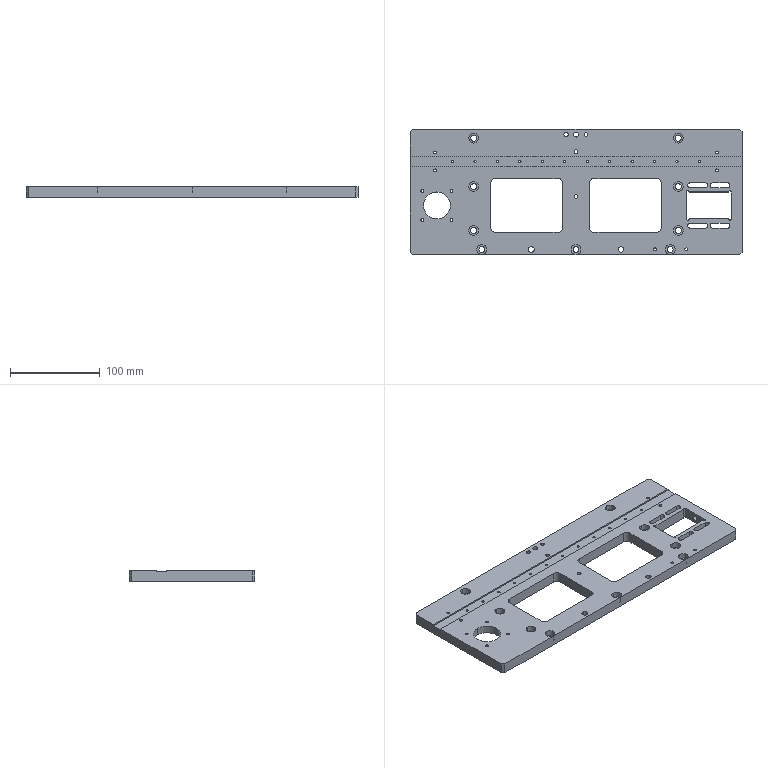CAM job | NX | 3-axis milling, drilling | part box 370 x 140 x 12 mm | stock box 376 x 146 x 13 mm
Tools:
number,name,description,diameter,corner_radius,flute_length,length,flutes
1,D50,Milling Tool-5 Parameters,50.0,0.0,50.0,75.0,2
3,D10,Milling Tool-5 Parameters,10.0,0.0,50.0,75.0,2
2,D6A45,Milling Tool-5 Parameters,6.0,0.0,3.0,3.0,2
13,3.3ZT,Drilling Tool,3.3,0.0,35.0,50.0,2
17,M4,Milling Tool-5 Parameters,3.3,0.0,30.0,30.0,4
14,4.2ZT,Drilling Tool,4.2,0.0,35.0,50.0,2
15,M5,Milling Tool-5 Parameters,4.2,0.0,30.0,30.0,4
16,6.6ZT,Drilling Tool,6.6,0.0,35.0,50.0,2
11,5.5ZT,Drilling Tool,5.5,0.0,35.0,50.0,2
12,2.5ZT,Drilling Tool,2.5,0.0,35.0,50.0,2
18,M3,Milling Tool-5 Parameters,2.5,0.0,30.0,30.0,4
8,D6,Milling Tool-5 Parameters,6.0,0.0,50.0,75.0,2
10,D4,Milling Tool-5 Parameters,4.0,0.0,50.0,75.0,2
20,D3,Milling Tool-5 Parameters,3.0,0.0,50.0,75.0,2
4,D10JING,Milling Tool-5 Parameters,10.0,0.0,50.0,75.0,2
Operations:
program,operation,operation_type,tool,method,geometry_group,spindle_rpm,surface_speed,feed_per_tooth,feed_cut,feed_plunge,cut_length_mm,path_length_mm,cut_time_min,machine_time_min
1-373-143-12-AB胶,FLOOR_WALL,VolumeBased25DMillingOperation,D50,METHOD,A,6500.0,1286.0,0.0962,1250.0,100.0,3119.997,3173.997,2.496,2.501
1-373-143-12-AB胶,ZLEVEL_PROFILE,ZLevelMilling,D10,METHOD,A,7000.0,219.0,0.2143,3000.0,1000.0,12643.007,12711.407,4.245,4.252
1-373-143-12-AB胶,FLOOR_WALL_2,VolumeBased25DMillingOperation,D10,METHOD,A,7500.0,235.0,0.1667,2500.0,1000.0,1542.469,1604.468,0.6216,0.6278
1-373-143-12-AB胶,ZLEVEL_PROFILE_COPY,ZLevelMilling,D10,METHOD,A,7000.0,219.0,0.2143,3000.0,1000.0,8316.956,9209.029,2.897,2.986
1-373-143-12-AB胶,DRILLING_COPY_1,Operation,D6A45,METHOD,A,3000.0,56.0,0.0333,200.0,0.0,179.4,1614.119,0.897,1.04
1-373-143-12-AB胶,DRILLING_COPY_1_COPY_COPY_COPY_COPY_COPY,Operation,3.3ZT,METHOD,A,2000.0,20.0,0.0375,150.0,0.0,162.914,939.211,1.086,1.164
1-373-143-12-AB胶,DRILLING_COPY_1_COPY_COPY_COPY_COPY_COPY_COPY_1,Operation,3.3ZT,METHOD,A,2000.0,20.0,0.0375,150.0,0.0,34.983,155.665,0.2332,0.2453
1-373-143-12-AB胶,DRILLING_COPY_1_COPY_COPY_COPY_COPY_COPY_COPY,Operation,M4,METHOD,A,200.0,2.0,0.175,140.0,0.0,143.0,899.383,1.021,1.097
1-373-143-12-AB胶,DRILLING_COPY_1_COPY,Operation,4.2ZT,METHOD,A,2000.0,15.0,0.0375,150.0,0.0,35.524,184.137,0.2368,0.2517
1-373-143-12-AB胶,DRILLING_COPY_1_COPY_COPY,Operation,M5,METHOD,A,200.0,2.0,0.2,160.0,0.0,31.0,175.09,0.1938,0.2082
1-373-143-12-AB胶,DRILLING_COPY_1_COPY_COPY_1_COPY_1,Operation,6.6ZT,METHOD,A,2000.0,18.0,0.03,120.0,0.0,166.346,879.214,1.386,1.458
1-373-143-12-AB胶,DRILLING_COPY_1_COPY_COPY_1_COPY_1_COPY,Operation,5.5ZT,METHOD,A,2000.0,18.0,0.03,120.0,0.0,52.957,410.093,0.4413,0.477
1-373-143-12-AB胶,DRILLING_COPY_1_COPY_1,Operation,2.5ZT,METHOD,A,2000.0,15.0,0.0375,150.0,0.0,189.013,750.999,1.26,1.316
1-373-143-12-AB胶,DRILLING_COPY_1_COPY_COPY_2,Operation,M3,METHOD,A,200.0,1.0,0.125,100.0,0.0,168.0,708.973,1.68,1.734
1-373-143-12-AB胶,HOLE_MILLING,CylinderMilling,D6,METHOD,A,7000.0,131.0,0.1071,1500.0,100.0,2163.975,3218.769,1.443,1.548
1-373-143-12-AB胶,ZLEVEL_PROFILE_COPY_1,ZLevelMilling,D4,METHOD,A,7000.0,87.0,0.1071,1500.0,1000.0,1053.265,1935.507,0.7466,0.8349
1-373-143-12-AB胶,ZLEVEL_PROFILE_COPY_2,ZLevelMilling,D4,METHOD,A,7000.0,87.0,0.1,1400.0,1000.0,6243.34,6611.81,4.499,4.536
1-373-143-12-AB胶,ZLEVEL_PROFILE_1,ZLevelMilling,D4,METHOD,A,7000.0,87.0,0.1071,1500.0,1000.0,587.57,828.086,0.4083,0.4323
1-373-143-12-AB胶,ZLEVEL_PROFILE_1_COPY,ZLevelMilling,D3,METHOD,A,7000.0,65.0,0.0714,1000.0,1000.0,464.656,625.356,0.4647,0.4807
1-373-143-12-AB胶,ZLEVEL_PROFILE_COPY_1_COPY,ZLevelMilling,D3,METHOD,A,7000.0,65.0,0.0929,1300.0,1000.0,734.718,1256.148,0.5947,0.6469
1-373-143-12-AB胶,FLOOR_WALL_1_COPY_1,VolumeBased25DMillingOperation,D10JING,METHOD,A,7000.0,87.0,0.0714,1000.0,100.0,1540.752,1604.452,1.541,1.547
1-373-143-12-AB胶,ZLEVEL_PROFILE_COPY_COPY_1_COPY_COPY_COPY_1,ZLevelMilling,D6,METHOD,A,7000.0,219.0,0.0714,1000.0,100.0,725.076,1354.562,0.7251,0.788
1-373-143-12-AB胶,ZLEVEL_PROFILE_COPY_1_COPY_COPY_COPY_COPY_2_COPY,ZLevelMilling,D6A45,METHOD,A,7000.0,131.0,0.0714,1000.0,1000.0,3166.445,11360.62,3.166,3.986
1-373-143-12-AB胶,刀补4,VolumeBased25DMillingOperation,D10JING,METHOD,A,7000.0,87.0,0.0714,1000.0,100.0,771.037,831.037,0.771,0.777
1-373-143-12-AB胶,刀补10,ZLevelMilling,D4,METHOD,A,7000.0,87.0,0.0607,850.0,1000.0,184.009,428.778,0.216,0.2405
1-373-143-12-AB胶,刀补10_COPY,ZLevelMilling,D3,METHOD,A,7000.0,87.0,0.0607,850.0,1000.0,105.212,270.697,0.1234,0.1399
1-373-143-12-AB胶,ZLEVEL_PROFILE_COPY_1_1,ZLevelMilling,D10JING,METHOD,A,7000.0,219.0,0.0714,1000.0,1000.0,3366.403,3437.153,3.366,3.373